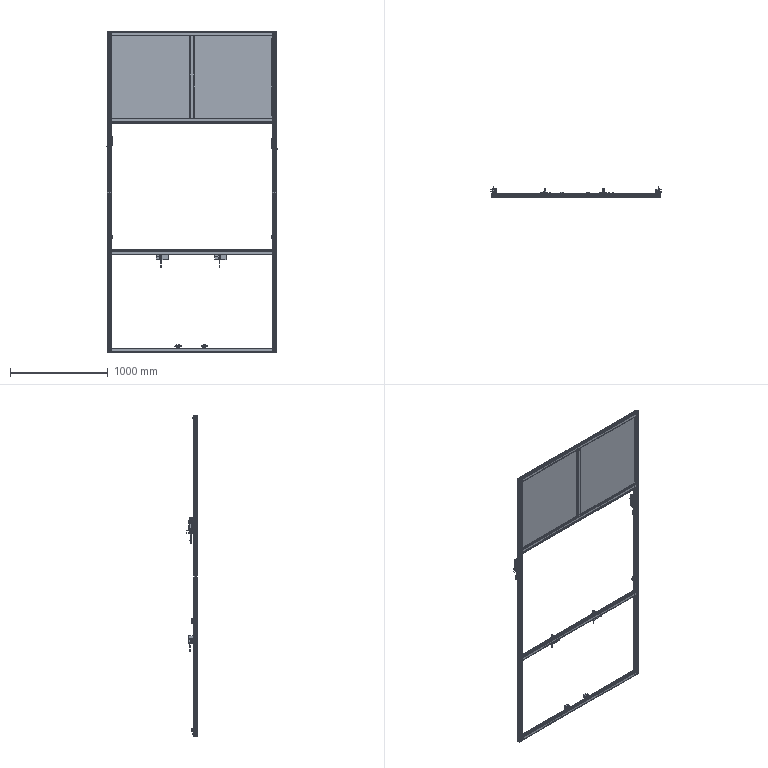Part | SolidWorks | features ReferencePattern 45, LocalLPattern 6, MirrorCompFeat 5, CompositeCurve 3 | 192 solids | 15492 faces | volume 16846770 mm3 | plane 8745 | cylinder 3557 | cone 1620 | spline 1160 | torus 322 | sphere 88 | commonest cylinder face diameters 2.5 x336 1 x306 2 x270 5 x214 6.8 x181 0.562 x180